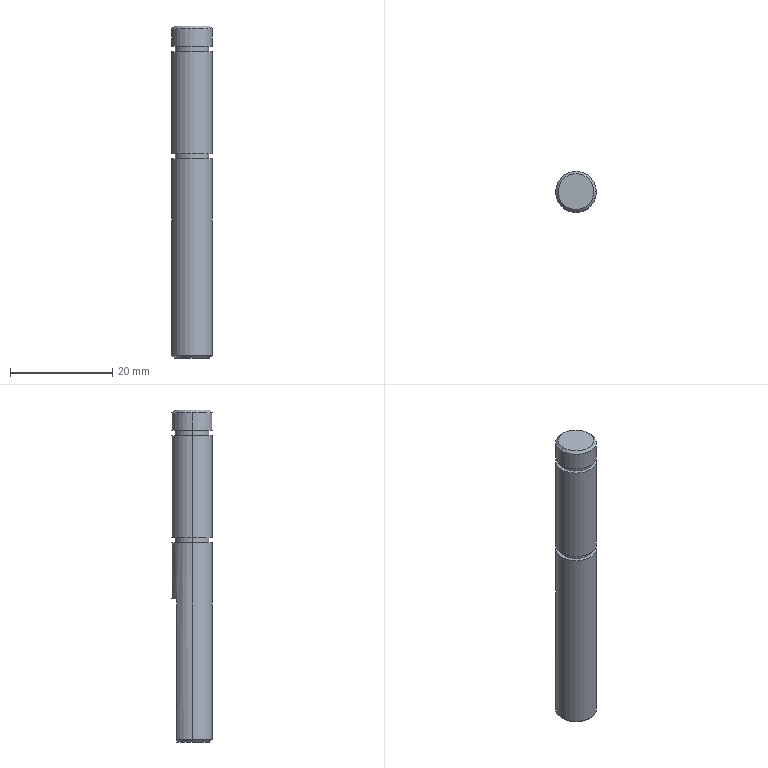Part | SolidWorks | features BaseBody 1 | 1 solid | 23 faces | box 8 x 8 x 65 mm | volume 3128 mm3 | cylinder 10 | plane 8 | cone 5 | commonest cylinder face diameters 8 x6 6.6 x4
STEP:
#1=CARTESIAN_POINT('',(3.5,0.,65.));
#2=VERTEX_POINT('',#1);
#3=CARTESIAN_POINT('',(4.,0.,64.5));
#4=VERTEX_POINT('',#3);
#5=CARTESIAN_POINT('',(3.5,0.,65.));
#6=DIRECTION('',(0.7071,0.,-0.7071));
#7=VECTOR('',#6,1000.);
#8=LINE('',#5,#7);
#9=EDGE_CURVE('',#2,#4,#8,.T.);
#10=ORIENTED_EDGE('',*,*,#9,.F.);
#11=CARTESIAN_POINT('',(-3.5,0.,65.));
#12=VERTEX_POINT('',#11);
#13=CARTESIAN_POINT('',(0.,0.,65.));
#14=DIRECTION('',(0.,0.,1.));
#15=DIRECTION('',(1.,0.,0.));
#16=AXIS2_PLACEMENT_3D('',#13,#14,#15);
#17=CIRCLE('',#16,3.5);
#18=EDGE_CURVE('',#12,#2,#17,.T.);
#19=ORIENTED_EDGE('',*,*,#18,.F.);
#20=CARTESIAN_POINT('',(-4.,0.,64.5));
#21=VERTEX_POINT('',#20);
#22=CARTESIAN_POINT('',(-3.5,0.,65.));
#23=DIRECTION('',(-0.7071,0.,-0.7071));
#24=VECTOR('',#23,1000.);
#25=LINE('',#22,#24);
#26=EDGE_CURVE('',#12,#21,#25,.T.);
#27=ORIENTED_EDGE('',*,*,#26,.T.);
#28=CARTESIAN_POINT('',(0.,0.,64.5));
#29=DIRECTION('',(0.,0.,-1.));
#30=DIRECTION('',(1.,0.,0.));
#31=AXIS2_PLACEMENT_3D('',#28,#29,#30);
#32=CIRCLE('',#31,4.);
#33=EDGE_CURVE('',#4,#21,#32,.T.);
#34=ORIENTED_EDGE('',*,*,#33,.F.);
#35=EDGE_LOOP('',(#10,#19,#27,#34));
#36=FACE_OUTER_BOUND('',#35,.T.);
#37=CARTESIAN_POINT('',(0.,0.,65.));
#38=DIRECTION('',(0.,0.,-1.));
#39=DIRECTION('',(-1.,0.,0.));
#40=AXIS2_PLACEMENT_3D('',#37,#38,#39);
#41=CONICAL_SURFACE('',#40,3.5,0.7854);
#42=ADVANCED_FACE('',(#36),#41,.T.);
#43=CARTESIAN_POINT('',(3.5,0.,0.));
#44=VERTEX_POINT('',#43);
#45=CARTESIAN_POINT('',(4.,0.,0.5));
#46=VERTEX_POINT('',#45);
#47=CARTESIAN_POINT('',(4.,0.,0.5));
#48=DIRECTION('',(0.7071,0.,0.7071));
#49=VECTOR('',#48,1000.);
#50=LINE('',#47,#49);
#51=EDGE_CURVE('',#44,#46,#50,.T.);
#52=ORIENTED_EDGE('',*,*,#51,.F.);
#53=CARTESIAN_POINT('',(1.803,3.,0.));
#54=VERTEX_POINT('',#53);
#55=CARTESIAN_POINT('',(0.,0.,0.));
#56=DIRECTION('',(0.,0.,-1.));
#57=DIRECTION('',(1.,0.,0.));
#58=AXIS2_PLACEMENT_3D('',#55,#56,#57);
#59=CIRCLE('',#58,3.5);
#60=EDGE_CURVE('',#54,#44,#59,.T.);
#61=ORIENTED_EDGE('',*,*,#60,.F.);
#62=CARTESIAN_POINT('',(2.646,3.,0.5));
#63=VERTEX_POINT('',#62);
#64=CARTESIAN_POINT('',(2.646,3.,0.5));
#65=CARTESIAN_POINT('',(2.346,3.,0.3018));
#66=CARTESIAN_POINT('',(2.065,3.,0.1351));
#67=CARTESIAN_POINT('',(1.803,3.,0.));
#68=B_SPLINE_CURVE_WITH_KNOTS('',3,(#64,#65,#66,#67),.UNSPECIFIED.,.F.,.F.,(4,4),(0.,1.),.UNSPECIFIED.);
#69=EDGE_CURVE('',#63,#54,#68,.T.);
#70=ORIENTED_EDGE('',*,*,#69,.F.);
#71=CARTESIAN_POINT('',(0.,0.,0.5));
#72=DIRECTION('',(0.,0.,1.));
#73=DIRECTION('',(1.,0.,0.));
#74=AXIS2_PLACEMENT_3D('',#71,#72,#73);
#75=CIRCLE('',#74,4.);
#76=EDGE_CURVE('',#46,#63,#75,.T.);
#77=ORIENTED_EDGE('',*,*,#76,.F.);
#78=EDGE_LOOP('',(#52,#61,#70,#77));
#79=FACE_OUTER_BOUND('',#78,.T.);
#80=CARTESIAN_POINT('',(0.,0.,0.5));
#81=DIRECTION('',(0.,0.,1.));
#82=DIRECTION('',(1.,0.,0.));
#83=AXIS2_PLACEMENT_3D('',#80,#81,#82);
#84=CONICAL_SURFACE('',#83,4.,0.7854);
#85=ADVANCED_FACE('',(#79),#84,.T.);
#86=CARTESIAN_POINT('',(-2.646,3.,28.));
#87=VERTEX_POINT('',#86);
#88=CARTESIAN_POINT('',(2.646,3.,28.));
#89=VERTEX_POINT('',#88);
#90=CARTESIAN_POINT('',(0.,0.,28.));
#91=DIRECTION('',(0.,0.,-1.));
#92=DIRECTION('',(-1.,0.,0.));
#93=AXIS2_PLACEMENT_3D('',#90,#91,#92);
#94=CIRCLE('',#93,4.);
#95=EDGE_CURVE('',#87,#89,#94,.T.);
#96=ORIENTED_EDGE('',*,*,#95,.T.);
#97=CARTESIAN_POINT('',(6.701,3.,28.));
#98=DIRECTION('',(-1.,0.,0.));
#99=VECTOR('',#98,1000.);
#100=LINE('',#97,#99);
#101=EDGE_CURVE('',#89,#87,#100,.T.);
#102=ORIENTED_EDGE('',*,*,#101,.T.);
#103=EDGE_LOOP('',(#96,#102));
#104=FACE_OUTER_BOUND('',#103,.T.);
#105=CARTESIAN_POINT('',(0.,0.,28.));
#106=DIRECTION('',(0.,0.,-1.));
#107=DIRECTION('',(0.,-1.,0.));
#108=AXIS2_PLACEMENT_3D('',#105,#106,#107);
#109=PLANE('',#108);
#110=ADVANCED_FACE('',(#104),#109,.T.);
#111=CARTESIAN_POINT('',(2.646,3.,65.));
#112=DIRECTION('',(0.,0.,1.));
#113=VECTOR('',#112,1000.);
#114=LINE('',#111,#113);
#115=EDGE_CURVE('',#63,#89,#114,.T.);
#116=ORIENTED_EDGE('',*,*,#115,.F.);
#117=ORIENTED_EDGE('',*,*,#69,.T.);
#118=CARTESIAN_POINT('',(-1.803,3.,0.));
#119=VERTEX_POINT('',#118);
#120=CARTESIAN_POINT('',(6.701,3.,0.));
#121=DIRECTION('',(-1.,0.,0.));
#122=VECTOR('',#121,1000.);
#123=LINE('',#120,#122);
#124=EDGE_CURVE('',#54,#119,#123,.T.);
#125=ORIENTED_EDGE('',*,*,#124,.T.);
#126=CARTESIAN_POINT('',(-2.646,3.,0.5));
#127=VERTEX_POINT('',#126);
#128=CARTESIAN_POINT('',(-1.803,3.,0.));
#129=CARTESIAN_POINT('',(-2.065,3.,0.1351));
#130=CARTESIAN_POINT('',(-2.346,3.,0.3018));
#131=CARTESIAN_POINT('',(-2.646,3.,0.5));
#132=B_SPLINE_CURVE_WITH_KNOTS('',3,(#128,#129,#130,#131),.UNSPECIFIED.,.F.,.F.,(4,4),(0.,1.),.UNSPECIFIED.);
#133=EDGE_CURVE('',#119,#127,#132,.T.);
#134=ORIENTED_EDGE('',*,*,#133,.T.);
#135=CARTESIAN_POINT('',(-2.646,3.,65.));
#136=DIRECTION('',(0.,0.,-1.));
#137=VECTOR('',#136,1000.);
#138=LINE('',#135,#137);
#139=EDGE_CURVE('',#87,#127,#138,.T.);
#140=ORIENTED_EDGE('',*,*,#139,.F.);
#141=ORIENTED_EDGE('',*,*,#101,.F.);
#142=EDGE_LOOP('',(#116,#117,#125,#134,#140,#141));
#143=FACE_OUTER_BOUND('',#142,.T.);
#144=CARTESIAN_POINT('',(6.701,3.,28.));
#145=DIRECTION('',(0.,-1.,0.));
#146=DIRECTION('',(0.,0.,-1.));
#147=AXIS2_PLACEMENT_3D('',#144,#145,#146);
#148=PLANE('',#147);
#149=ADVANCED_FACE('',(#143),#148,.F.);
#150=CARTESIAN_POINT('',(4.,0.,39.));
#151=VERTEX_POINT('',#150);
#152=CARTESIAN_POINT('',(4.,0.,65.));
#153=DIRECTION('',(0.,0.,-1.));
#154=VECTOR('',#153,1000.);
#155=LINE('',#152,#154);
#156=EDGE_CURVE('',#151,#46,#155,.T.);
#157=ORIENTED_EDGE('',*,*,#156,.F.);
#158=CARTESIAN_POINT('',(-4.,0.,39.));
#159=VERTEX_POINT('',#158);
#160=CARTESIAN_POINT('',(0.,0.,39.));
#161=DIRECTION('',(0.,0.,-1.));
#162=DIRECTION('',(-1.,0.,0.));
#163=AXIS2_PLACEMENT_3D('',#160,#161,#162);
#164=CIRCLE('',#163,4.);
#165=EDGE_CURVE('',#151,#159,#164,.T.);
#166=ORIENTED_EDGE('',*,*,#165,.T.);
#167=CARTESIAN_POINT('',(-4.,0.,0.5));
#168=VERTEX_POINT('',#167);
#169=CARTESIAN_POINT('',(-4.,0.,65.));
#170=DIRECTION('',(0.,0.,-1.));
#171=VECTOR('',#170,1000.);
#172=LINE('',#169,#171);
#173=EDGE_CURVE('',#159,#168,#172,.T.);
#174=ORIENTED_EDGE('',*,*,#173,.T.);
#175=CARTESIAN_POINT('',(0.,0.,0.5));
#176=DIRECTION('',(0.,0.,1.));
#177=DIRECTION('',(1.,0.,0.));
#178=AXIS2_PLACEMENT_3D('',#175,#176,#177);
#179=CIRCLE('',#178,4.);
#180=EDGE_CURVE('',#168,#46,#179,.T.);
#181=ORIENTED_EDGE('',*,*,#180,.T.);
#182=EDGE_LOOP('',(#157,#166,#174,#181));
#183=FACE_OUTER_BOUND('',#182,.T.);
#184=CARTESIAN_POINT('',(0.,0.,65.));
#185=DIRECTION('',(0.,0.,-1.));
#186=DIRECTION('',(-1.,0.,0.));
#187=AXIS2_PLACEMENT_3D('',#184,#185,#186);
#188=CYLINDRICAL_SURFACE('',#187,4.);
#189=ADVANCED_FACE('',(#183),#188,.T.);
#190=ORIENTED_EDGE('',*,*,#124,.F.);
#191=ORIENTED_EDGE('',*,*,#60,.T.);
#192=CARTESIAN_POINT('',(-3.5,0.,0.));
#193=VERTEX_POINT('',#192);
#194=CARTESIAN_POINT('',(0.,0.,0.));
#195=DIRECTION('',(0.,0.,-1.));
#196=DIRECTION('',(1.,0.,0.));
#197=AXIS2_PLACEMENT_3D('',#194,#195,#196);
#198=CIRCLE('',#197,3.5);
#199=EDGE_CURVE('',#44,#193,#198,.T.);
#200=ORIENTED_EDGE('',*,*,#199,.T.);
#201=CARTESIAN_POINT('',(0.,0.,0.));
#202=DIRECTION('',(0.,0.,-1.));
#203=DIRECTION('',(1.,0.,0.));
#204=AXIS2_PLACEMENT_3D('',#201,#202,#203);
#205=CIRCLE('',#204,3.5);
#206=EDGE_CURVE('',#193,#119,#205,.T.);
#207=ORIENTED_EDGE('',*,*,#206,.T.);
#208=EDGE_LOOP('',(#190,#191,#200,#207));
#209=FACE_OUTER_BOUND('',#208,.T.);
#210=CARTESIAN_POINT('',(0.,0.,0.));
#211=DIRECTION('',(0.,0.,1.));
#212=DIRECTION('',(1.,0.,0.));
#213=AXIS2_PLACEMENT_3D('',#210,#211,#212);
#214=PLANE('',#213);
#215=ADVANCED_FACE('',(#209),#214,.F.);
#216=CARTESIAN_POINT('',(-3.3,0.,39.));
#217=VERTEX_POINT('',#216);
#218=CARTESIAN_POINT('',(3.3,0.,39.));
#219=VERTEX_POINT('',#218);
#220=CARTESIAN_POINT('',(0.,0.,39.));
#221=DIRECTION('',(0.,0.,-1.));
#222=DIRECTION('',(-1.,0.,0.));
#223=AXIS2_PLACEMENT_3D('',#220,#221,#222);
#224=CIRCLE('',#223,3.3);
#225=EDGE_CURVE('',#217,#219,#224,.T.);
#226=ORIENTED_EDGE('',*,*,#225,.T.);
#227=CARTESIAN_POINT('',(0.,0.,39.));
#228=DIRECTION('',(0.,0.,-1.));
#229=DIRECTION('',(-1.,0.,0.));
#230=AXIS2_PLACEMENT_3D('',#227,#228,#229);
#231=CIRCLE('',#230,3.3);
#232=EDGE_CURVE('',#219,#217,#231,.T.);
#233=ORIENTED_EDGE('',*,*,#232,.T.);
#234=EDGE_LOOP('',(#226,#233));
#235=FACE_BOUND('',#234,.T.);
#236=CARTESIAN_POINT('',(0.,0.,39.));
#237=DIRECTION('',(0.,0.,-1.));
#238=DIRECTION('',(-1.,0.,0.));
#239=AXIS2_PLACEMENT_3D('',#236,#237,#238);
#240=CIRCLE('',#239,4.);
#241=EDGE_CURVE('',#159,#151,#240,.T.);
#242=ORIENTED_EDGE('',*,*,#241,.F.);
#243=ORIENTED_EDGE('',*,*,#165,.F.);
#244=EDGE_LOOP('',(#242,#243));
#245=FACE_OUTER_BOUND('',#244,.T.);
#246=CARTESIAN_POINT('',(0.,4.,39.));
#247=DIRECTION('',(0.,0.,-1.));
#248=DIRECTION('',(0.,-1.,0.));
#249=AXIS2_PLACEMENT_3D('',#246,#247,#248);
#250=PLANE('',#249);
#251=ADVANCED_FACE('',(#235,#245),#250,.F.);
#252=CARTESIAN_POINT('',(3.3,0.,40.));
#253=VERTEX_POINT('',#252);
#254=CARTESIAN_POINT('',(3.3,0.,65.));
#255=DIRECTION('',(0.,0.,-1.));
#256=VECTOR('',#255,1000.);
#257=LINE('',#254,#256);
#258=EDGE_CURVE('',#253,#219,#257,.T.);
#259=ORIENTED_EDGE('',*,*,#258,.F.);
#260=CARTESIAN_POINT('',(-3.3,0.,40.));
#261=VERTEX_POINT('',#260);
#262=CARTESIAN_POINT('',(0.,0.,40.));
#263=DIRECTION('',(0.,0.,-1.));
#264=DIRECTION('',(-1.,0.,0.));
#265=AXIS2_PLACEMENT_3D('',#262,#263,#264);
#266=CIRCLE('',#265,3.3);
#267=EDGE_CURVE('',#253,#261,#266,.T.);
#268=ORIENTED_EDGE('',*,*,#267,.T.);
#269=CARTESIAN_POINT('',(-3.3,0.,65.));
#270=DIRECTION('',(0.,0.,-1.));
#271=VECTOR('',#270,1000.);
#272=LINE('',#269,#271);
#273=EDGE_CURVE('',#261,#217,#272,.T.);
#274=ORIENTED_EDGE('',*,*,#273,.T.);
#275=ORIENTED_EDGE('',*,*,#232,.F.);
#276=EDGE_LOOP('',(#259,#268,#274,#275));
#277=FACE_OUTER_BOUND('',#276,.T.);
#278=CARTESIAN_POINT('',(0.,0.,65.));
#279=DIRECTION('',(0.,0.,-1.));
#280=DIRECTION('',(-1.,0.,0.));
#281=AXIS2_PLACEMENT_3D('',#278,#279,#280);
#282=CYLINDRICAL_SURFACE('',#281,3.3);
#283=ADVANCED_FACE('',(#277),#282,.T.);
#284=CARTESIAN_POINT('',(0.,0.,40.));
#285=DIRECTION('',(0.,0.,-1.));
#286=DIRECTION('',(-1.,0.,0.));
#287=AXIS2_PLACEMENT_3D('',#284,#285,#286);
#288=CIRCLE('',#287,3.3);
#289=EDGE_CURVE('',#261,#253,#288,.T.);
#290=ORIENTED_EDGE('',*,*,#289,.F.);
#291=ORIENTED_EDGE('',*,*,#267,.F.);
#292=EDGE_LOOP('',(#290,#291));
#293=FACE_BOUND('',#292,.T.);
#294=CARTESIAN_POINT('',(-4.,0.,40.));
#295=VERTEX_POINT('',#294);
#296=CARTESIAN_POINT('',(4.,0.,40.));
#297=VERTEX_POINT('',#296);
#298=CARTESIAN_POINT('',(0.,0.,40.));
#299=DIRECTION('',(0.,0.,-1.));
#300=DIRECTION('',(-1.,0.,0.));
#301=AXIS2_PLACEMENT_3D('',#298,#299,#300);
#302=CIRCLE('',#301,4.);
#303=EDGE_CURVE('',#295,#297,#302,.T.);
#304=ORIENTED_EDGE('',*,*,#303,.T.);
#305=CARTESIAN_POINT('',(0.,0.,40.));
#306=DIRECTION('',(0.,0.,-1.));
#307=DIRECTION('',(-1.,0.,0.));
#308=AXIS2_PLACEMENT_3D('',#305,#306,#307);
#309=CIRCLE('',#308,4.);
#310=EDGE_CURVE('',#297,#295,#309,.T.);
#311=ORIENTED_EDGE('',*,*,#310,.T.);
#312=EDGE_LOOP('',(#304,#311));
#313=FACE_OUTER_BOUND('',#312,.T.);
#314=CARTESIAN_POINT('',(0.,4.,40.));
#315=DIRECTION('',(0.,0.,1.));
#316=DIRECTION('',(1.,0.,0.));
#317=AXIS2_PLACEMENT_3D('',#314,#315,#316);
#318=PLANE('',#317);
#319=ADVANCED_FACE('',(#293,#313),#318,.F.);
#320=CARTESIAN_POINT('',(4.,0.,60.));
#321=VERTEX_POINT('',#320);
#322=CARTESIAN_POINT('',(4.,0.,65.));
#323=DIRECTION('',(0.,0.,-1.));
#324=VECTOR('',#323,1000.);
#325=LINE('',#322,#324);
#326=EDGE_CURVE('',#321,#297,#325,.T.);
#327=ORIENTED_EDGE('',*,*,#326,.F.);
#328=CARTESIAN_POINT('',(-4.,0.,60.));
#329=VERTEX_POINT('',#328);
#330=CARTESIAN_POINT('',(0.,0.,60.));
#331=DIRECTION('',(0.,0.,-1.));
#332=DIRECTION('',(-1.,0.,0.));
#333=AXIS2_PLACEMENT_3D('',#330,#331,#332);
#334=CIRCLE('',#333,4.);
#335=EDGE_CURVE('',#321,#329,#334,.T.);
#336=ORIENTED_EDGE('',*,*,#335,.T.);
#337=CARTESIAN_POINT('',(-4.,0.,65.));
#338=DIRECTION('',(0.,0.,-1.));
#339=VECTOR('',#338,1000.);
#340=LINE('',#337,#339);
#341=EDGE_CURVE('',#329,#295,#340,.T.);
#342=ORIENTED_EDGE('',*,*,#341,.T.);
#343=ORIENTED_EDGE('',*,*,#310,.F.);
#344=EDGE_LOOP('',(#327,#336,#342,#343));
#345=FACE_OUTER_BOUND('',#344,.T.);
#346=CARTESIAN_POINT('',(0.,0.,65.));
#347=DIRECTION('',(0.,0.,-1.));
#348=DIRECTION('',(-1.,0.,0.));
#349=AXIS2_PLACEMENT_3D('',#346,#347,#348);
#350=CYLINDRICAL_SURFACE('',#349,4.);
#351=ADVANCED_FACE('',(#345),#350,.T.);
#352=CARTESIAN_POINT('',(-3.3,0.,60.));
#353=VERTEX_POINT('',#352);
#354=CARTESIAN_POINT('',(3.3,0.,60.));
#355=VERTEX_POINT('',#354);
#356=CARTESIAN_POINT('',(0.,0.,60.));
#357=DIRECTION('',(0.,0.,-1.));
#358=DIRECTION('',(-1.,0.,0.));
#359=AXIS2_PLACEMENT_3D('',#356,#357,#358);
#360=CIRCLE('',#359,3.3);
#361=EDGE_CURVE('',#353,#355,#360,.T.);
#362=ORIENTED_EDGE('',*,*,#361,.T.);
#363=CARTESIAN_POINT('',(0.,0.,60.));
#364=DIRECTION('',(0.,0.,-1.));
#365=DIRECTION('',(-1.,0.,0.));
#366=AXIS2_PLACEMENT_3D('',#363,#364,#365);
#367=CIRCLE('',#366,3.3);
#368=EDGE_CURVE('',#355,#353,#367,.T.);
#369=ORIENTED_EDGE('',*,*,#368,.T.);
#370=EDGE_LOOP('',(#362,#369));
#371=FACE_BOUND('',#370,.T.);
#372=CARTESIAN_POINT('',(0.,0.,60.));
#373=DIRECTION('',(0.,0.,-1.));
#374=DIRECTION('',(-1.,0.,0.));
#375=AXIS2_PLACEMENT_3D('',#372,#373,#374);
#376=CIRCLE('',#375,4.);
#377=EDGE_CURVE('',#329,#321,#376,.T.);
#378=ORIENTED_EDGE('',*,*,#377,.F.);
#379=ORIENTED_EDGE('',*,*,#335,.F.);
#380=EDGE_LOOP('',(#378,#379));
#381=FACE_OUTER_BOUND('',#380,.T.);
#382=CARTESIAN_POINT('',(0.,4.,60.));
#383=DIRECTION('',(0.,0.,-1.));
#384=DIRECTION('',(0.,-1.,0.));
#385=AXIS2_PLACEMENT_3D('',#382,#383,#384);
#386=PLANE('',#385);
#387=ADVANCED_FACE('',(#371,#381),#386,.F.);
#388=CARTESIAN_POINT('',(3.3,0.,61.));
#389=VERTEX_POINT('',#388);
#390=CARTESIAN_POINT('',(3.3,0.,65.));
#391=DIRECTION('',(0.,0.,-1.));
#392=VECTOR('',#391,1000.);
#393=LINE('',#390,#392);
#394=EDGE_CURVE('',#389,#355,#393,.T.);
#395=ORIENTED_EDGE('',*,*,#394,.F.);
#396=CARTESIAN_POINT('',(-3.3,0.,61.));
#397=VERTEX_POINT('',#396);
#398=CARTESIAN_POINT('',(0.,0.,61.));
#399=DIRECTION('',(0.,0.,-1.));
#400=DIRECTION('',(-1.,0.,0.));
#401=AXIS2_PLACEMENT_3D('',#398,#399,#400);
#402=CIRCLE('',#401,3.3);
#403=EDGE_CURVE('',#389,#397,#402,.T.);
#404=ORIENTED_EDGE('',*,*,#403,.T.);
#405=CARTESIAN_POINT('',(-3.3,0.,65.));
#406=DIRECTION('',(0.,0.,-1.));
#407=VECTOR('',#406,1000.);
#408=LINE('',#405,#407);
#409=EDGE_CURVE('',#397,#353,#408,.T.);
#410=ORIENTED_EDGE('',*,*,#409,.T.);
#411=ORIENTED_EDGE('',*,*,#368,.F.);
#412=EDGE_LOOP('',(#395,#404,#410,#411));
#413=FACE_OUTER_BOUND('',#412,.T.);
#414=CARTESIAN_POINT('',(0.,0.,65.));
#415=DIRECTION('',(0.,0.,-1.));
#416=DIRECTION('',(-1.,0.,0.));
#417=AXIS2_PLACEMENT_3D('',#414,#415,#416);
#418=CYLINDRICAL_SURFACE('',#417,3.3);
#419=ADVANCED_FACE('',(#413),#418,.T.);
#420=CARTESIAN_POINT('',(0.,0.,61.));
#421=DIRECTION('',(0.,0.,-1.));
#422=DIRECTION('',(-1.,0.,0.));
#423=AXIS2_PLACEMENT_3D('',#420,#421,#422);
#424=CIRCLE('',#423,3.3);
#425=EDGE_CURVE('',#397,#389,#424,.T.);
#426=ORIENTED_EDGE('',*,*,#425,.F.);
#427=ORIENTED_EDGE('',*,*,#403,.F.);
#428=EDGE_LOOP('',(#426,#427));
#429=FACE_BOUND('',#428,.T.);
#430=CARTESIAN_POINT('',(-4.,0.,61.));
#431=VERTEX_POINT('',#430);
#432=CARTESIAN_POINT('',(4.,0.,61.));
#433=VERTEX_POINT('',#432);
#434=CARTESIAN_POINT('',(0.,0.,61.));
#435=DIRECTION('',(0.,0.,-1.));
#436=DIRECTION('',(-1.,0.,0.));
#437=AXIS2_PLACEMENT_3D('',#434,#435,#436);
#438=CIRCLE('',#437,4.);
#439=EDGE_CURVE('',#431,#433,#438,.T.);
#440=ORIENTED_EDGE('',*,*,#439,.T.);
#441=CARTESIAN_POINT('',(0.,0.,61.));
#442=DIRECTION('',(0.,0.,-1.));
#443=DIRECTION('',(-1.,0.,0.));
#444=AXIS2_PLACEMENT_3D('',#441,#442,#443);
#445=CIRCLE('',#444,4.);
#446=EDGE_CURVE('',#433,#431,#445,.T.);
#447=ORIENTED_EDGE('',*,*,#446,.T.);
#448=EDGE_LOOP('',(#440,#447));
#449=FACE_OUTER_BOUND('',#448,.T.);
#450=CARTESIAN_POINT('',(0.,4.,61.));
#451=DIRECTION('',(0.,0.,1.));
#452=DIRECTION('',(1.,0.,0.));
#453=AXIS2_PLACEMENT_3D('',#450,#451,#452);
#454=PLANE('',#453);
#455=ADVANCED_FACE('',(#429,#449),#454,.F.);
#456=ORIENTED_EDGE('',*,*,#18,.T.);
#457=CARTESIAN_POINT('',(0.,0.,65.));
#458=DIRECTION('',(0.,0.,1.));
#459=DIRECTION('',(1.,0.,0.));
#460=AXIS2_PLACEMENT_3D('',#457,#458,#459);
#461=CIRCLE('',#460,3.5);
#462=EDGE_CURVE('',#2,#12,#461,.T.);
#463=ORIENTED_EDGE('',*,*,#462,.T.);
#464=EDGE_LOOP('',(#456,#463));
#465=FACE_OUTER_BOUND('',#464,.T.);
#466=CARTESIAN_POINT('',(0.,0.,65.));
#467=DIRECTION('',(0.,0.,1.));
#468=DIRECTION('',(1.,0.,0.));
#469=AXIS2_PLACEMENT_3D('',#466,#467,#468);
#470=PLANE('',#469);
#471=ADVANCED_FACE('',(#465),#470,.T.);
#472=CARTESIAN_POINT('',(4.,0.,65.));
#473=DIRECTION('',(0.,0.,-1.));
#474=VECTOR('',#473,1000.);
#475=LINE('',#472,#474);
#476=EDGE_CURVE('',#4,#433,#475,.T.);
#477=ORIENTED_EDGE('',*,*,#476,.F.);
#478=ORIENTED_EDGE('',*,*,#33,.T.);
#479=CARTESIAN_POINT('',(-4.,0.,65.));
#480=DIRECTION('',(0.,0.,-1.));
#481=VECTOR('',#480,1000.);
#482=LINE('',#479,#481);
#483=EDGE_CURVE('',#21,#431,#482,.T.);
#484=ORIENTED_EDGE('',*,*,#483,.T.);
#485=ORIENTED_EDGE('',*,*,#446,.F.);
#486=EDGE_LOOP('',(#477,#478,#484,#485));
#487=FACE_OUTER_BOUND('',#486,.T.);
#488=CARTESIAN_POINT('',(0.,0.,65.));
#489=DIRECTION('',(0.,0.,-1.));
#490=DIRECTION('',(-1.,0.,0.));
#491=AXIS2_PLACEMENT_3D('',#488,#489,#490);
#492=CYLINDRICAL_SURFACE('',#491,4.);
#493=ADVANCED_FACE('',(#487),#492,.T.);
#494=CARTESIAN_POINT('',(0.,0.,64.5));
#495=DIRECTION('',(0.,0.,-1.));
#496=DIRECTION('',(1.,0.,0.));
#497=AXIS2_PLACEMENT_3D('',#494,#495,#496);
#498=CIRCLE('',#497,4.);
#499=EDGE_CURVE('',#21,#4,#498,.T.);
#500=ORIENTED_EDGE('',*,*,#499,.T.);
#501=ORIENTED_EDGE('',*,*,#476,.T.);
#502=ORIENTED_EDGE('',*,*,#439,.F.);
#503=ORIENTED_EDGE('',*,*,#483,.F.);
#504=EDGE_LOOP('',(#500,#501,#502,#503));
#505=FACE_OUTER_BOUND('',#504,.T.);
#506=CARTESIAN_POINT('',(0.,0.,65.));
#507=DIRECTION('',(0.,0.,-1.));
#508=DIRECTION('',(-1.,0.,0.));
#509=AXIS2_PLACEMENT_3D('',#506,#507,#508);
#510=CYLINDRICAL_SURFACE('',#509,4.);
#511=ADVANCED_FACE('',(#505),#510,.T.);
#512=ORIENTED_EDGE('',*,*,#425,.T.);
#513=ORIENTED_EDGE('',*,*,#394,.T.);
#514=ORIENTED_EDGE('',*,*,#361,.F.);
#515=ORIENTED_EDGE('',*,*,#409,.F.);
#516=EDGE_LOOP('',(#512,#513,#514,#515));
#517=FACE_OUTER_BOUND('',#516,.T.);
#518=CARTESIAN_POINT('',(0.,0.,65.));
#519=DIRECTION('',(0.,0.,-1.));
#520=DIRECTION('',(-1.,0.,0.));
#521=AXIS2_PLACEMENT_3D('',#518,#519,#520);
#522=CYLINDRICAL_SURFACE('',#521,3.3);
#523=ADVANCED_FACE('',(#517),#522,.T.);
#524=ORIENTED_EDGE('',*,*,#377,.T.);
#525=ORIENTED_EDGE('',*,*,#326,.T.);
#526=ORIENTED_EDGE('',*,*,#303,.F.);
#527=ORIENTED_EDGE('',*,*,#341,.F.);
#528=EDGE_LOOP('',(#524,#525,#526,#527));
#529=FACE_OUTER_BOUND('',#528,.T.);
#530=CARTESIAN_POINT('',(0.,0.,65.));
#531=DIRECTION('',(0.,0.,-1.));
#532=DIRECTION('',(-1.,0.,0.));
#533=AXIS2_PLACEMENT_3D('',#530,#531,#532);
#534=CYLINDRICAL_SURFACE('',#533,4.);
#535=ADVANCED_FACE('',(#529),#534,.T.);
#536=ORIENTED_EDGE('',*,*,#289,.T.);
#537=ORIENTED_EDGE('',*,*,#258,.T.);
#538=ORIENTED_EDGE('',*,*,#225,.F.);
#539=ORIENTED_EDGE('',*,*,#273,.F.);
#540=EDGE_LOOP('',(#536,#537,#538,#539));
#541=FACE_OUTER_BOUND('',#540,.T.);
#542=CARTESIAN_POINT('',(0.,0.,65.));
#543=DIRECTION('',(0.,0.,-1.));
#544=DIRECTION('',(-1.,0.,0.));
#545=AXIS2_PLACEMENT_3D('',#542,#543,#544);
#546=CYLINDRICAL_SURFACE('',#545,3.3);
#547=ADVANCED_FACE('',(#541),#546,.T.);
#548=ORIENTED_EDGE('',*,*,#241,.T.);
#549=ORIENTED_EDGE('',*,*,#156,.T.);
#550=ORIENTED_EDGE('',*,*,#76,.T.);
#551=ORIENTED_EDGE('',*,*,#115,.T.);
#552=ORIENTED_EDGE('',*,*,#95,.F.);
#553=ORIENTED_EDGE('',*,*,#139,.T.);
#554=CARTESIAN_POINT('',(0.,0.,0.5));
#555=DIRECTION('',(0.,0.,1.));
#556=DIRECTION('',(1.,0.,0.));
#557=AXIS2_PLACEMENT_3D('',#554,#555,#556);
#558=CIRCLE('',#557,4.);
#559=EDGE_CURVE('',#127,#168,#558,.T.);
#560=ORIENTED_EDGE('',*,*,#559,.T.);
#561=ORIENTED_EDGE('',*,*,#173,.F.);
#562=EDGE_LOOP('',(#548,#549,#550,#551,#552,#553,#560,#561));
#563=FACE_OUTER_BOUND('',#562,.T.);
#564=CARTESIAN_POINT('',(0.,0.,65.));
#565=DIRECTION('',(0.,0.,-1.));
#566=DIRECTION('',(-1.,0.,0.));
#567=AXIS2_PLACEMENT_3D('',#564,#565,#566);
#568=CYLINDRICAL_SURFACE('',#567,4.);
#569=ADVANCED_FACE('',(#563),#568,.T.);
#570=CARTESIAN_POINT('',(-4.,0.,0.5));
#571=DIRECTION('',(-0.7071,0.,0.7071));
#572=VECTOR('',#571,1000.);
#573=LINE('',#570,#572);
#574=EDGE_CURVE('',#193,#168,#573,.T.);
#575=ORIENTED_EDGE('',*,*,#574,.F.);
#576=ORIENTED_EDGE('',*,*,#199,.F.);
#577=ORIENTED_EDGE('',*,*,#51,.T.);
#578=ORIENTED_EDGE('',*,*,#180,.F.);
#579=EDGE_LOOP('',(#575,#576,#577,#578));
#580=FACE_OUTER_BOUND('',#579,.T.);
#581=CARTESIAN_POINT('',(0.,0.,0.5));
#582=DIRECTION('',(0.,0.,1.));
#583=DIRECTION('',(1.,0.,0.));
#584=AXIS2_PLACEMENT_3D('',#581,#582,#583);
#585=CONICAL_SURFACE('',#584,4.,0.7854);
#586=ADVANCED_FACE('',(#580),#585,.T.);
#587=ORIENTED_EDGE('',*,*,#206,.F.);
#588=ORIENTED_EDGE('',*,*,#574,.T.);
#589=ORIENTED_EDGE('',*,*,#559,.F.);
#590=ORIENTED_EDGE('',*,*,#133,.F.);
#591=EDGE_LOOP('',(#587,#588,#589,#590));
#592=FACE_OUTER_BOUND('',#591,.T.);
#593=CARTESIAN_POINT('',(0.,0.,0.5));
#594=DIRECTION('',(0.,0.,1.));
#595=DIRECTION('',(1.,0.,0.));
#596=AXIS2_PLACEMENT_3D('',#593,#594,#595);
#597=CONICAL_SURFACE('',#596,4.,0.7854);
#598=ADVANCED_FACE('',(#592),#597,.T.);
#599=ORIENTED_EDGE('',*,*,#462,.F.);
#600=ORIENTED_EDGE('',*,*,#9,.T.);
#601=ORIENTED_EDGE('',*,*,#499,.F.);
#602=ORIENTED_EDGE('',*,*,#26,.F.);
#603=EDGE_LOOP('',(#599,#600,#601,#602));
#604=FACE_OUTER_BOUND('',#603,.T.);
#605=CARTESIAN_POINT('',(0.,0.,65.));
#606=DIRECTION('',(0.,0.,-1.));
#607=DIRECTION('',(-1.,0.,0.));
#608=AXIS2_PLACEMENT_3D('',#605,#606,#607);
#609=CONICAL_SURFACE('',#608,3.5,0.7854);
#610=ADVANCED_FACE('',(#604),#609,.T.);
#611=CLOSED_SHELL('',(#42,#85,#110,#149,#189,#215,#251,#283,#319,#351,#387,#419,#455,#471,#493,#511,#523,#535,#547,#569,#586,#598,#610));
#612=MANIFOLD_SOLID_BREP('',#611);
#613=CARTESIAN_POINT('',(0.,0.,0.));
#614=DIRECTION('',(0.,0.,1.));
#615=DIRECTION('',(1.,0.,0.));
#616=AXIS2_PLACEMENT_3D('',#613,#614,#615);
#617=(LENGTH_UNIT()NAMED_UNIT(*)SI_UNIT(.MILLI.,.METRE.));
#618=UNCERTAINTY_MEASURE_WITH_UNIT(LENGTH_MEASURE(0.00001),#617,'','');
#619=(NAMED_UNIT(*)PLANE_ANGLE_UNIT()SI_UNIT($,.RADIAN.));
#620=(NAMED_UNIT(*)SI_UNIT($,.STERADIAN.)SOLID_ANGLE_UNIT());
#621=(GEOMETRIC_REPRESENTATION_CONTEXT(3)GLOBAL_UNCERTAINTY_ASSIGNED_CONTEXT((#618))GLOBAL_UNIT_ASSIGNED_CONTEXT((#617,#619,#620))REPRESENTATION_CONTEXT('',''));
#622=ADVANCED_BREP_SHAPE_REPRESENTATION('',(#612,#616),#621);